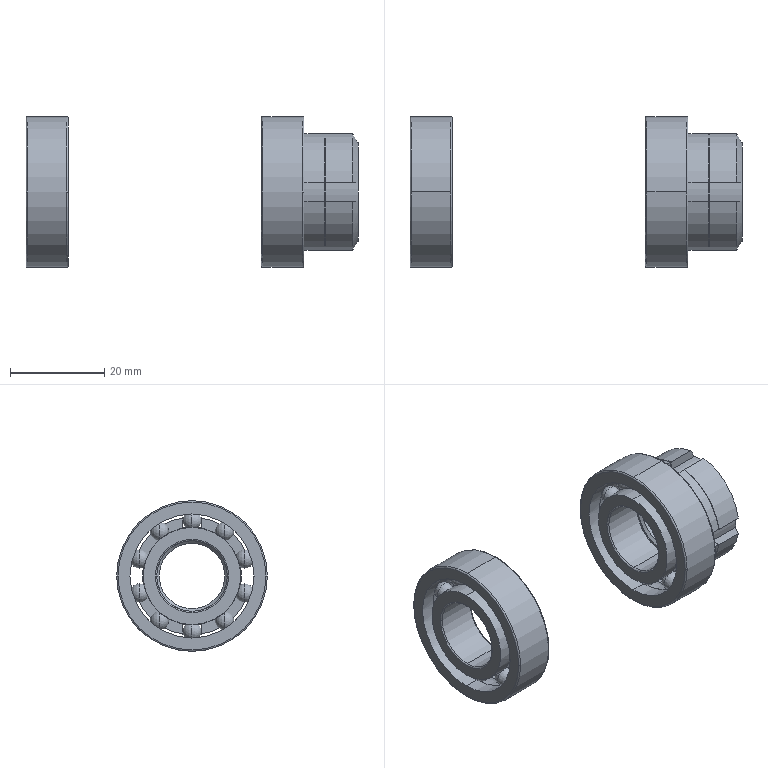Part | NX | 3 solids | 235 faces | box 70.5 x 32 x 32 mm | volume 11279 mm3 | torus 82 | cylinder 48 | plane 45 | sphere 40 | cone 20 | commonest cylinder face diameters 20.667 x8 21 x8 25 x8 26.333 x8 13.917 x4 15 x4